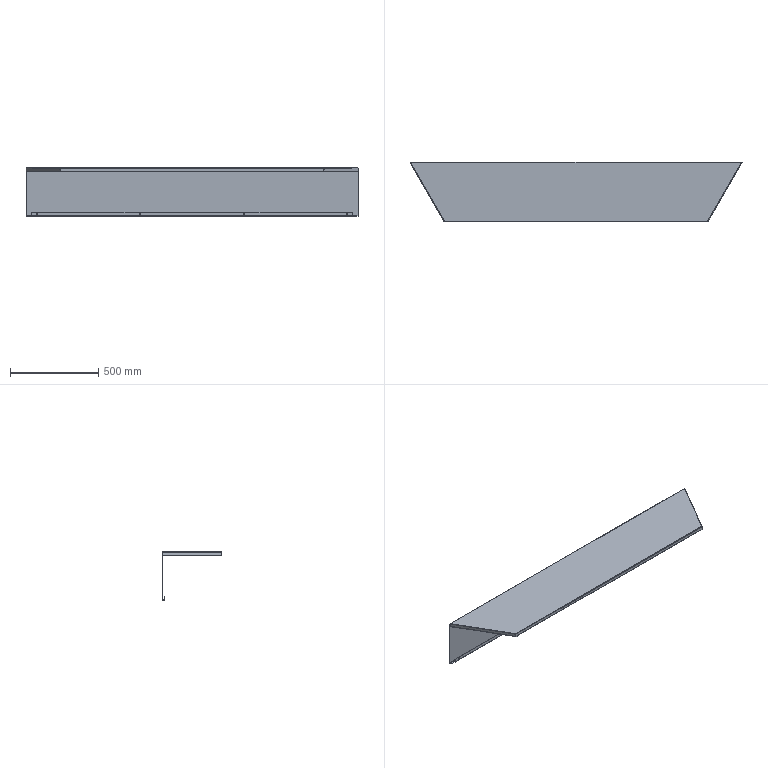Part | SolidWorks | features ICE 8, EdgeFlange 6, SMBaseFlange 5, SMMiteredFlange 2, FlatPattern 1, SheetMetal 1 | 1 solid | 151 faces | box 1885 x 336.9 x 273 mm | volume 1826006 mm3 | plane 111 | cylinder 38 | spline 2 | commonest cylinder face diameters 6.4 x20 1 x9 4 x9